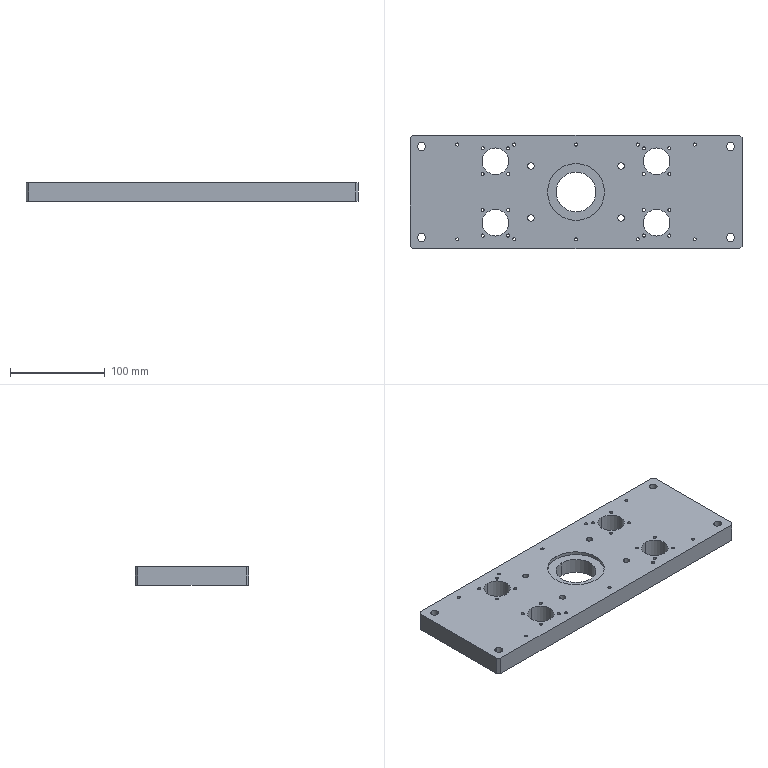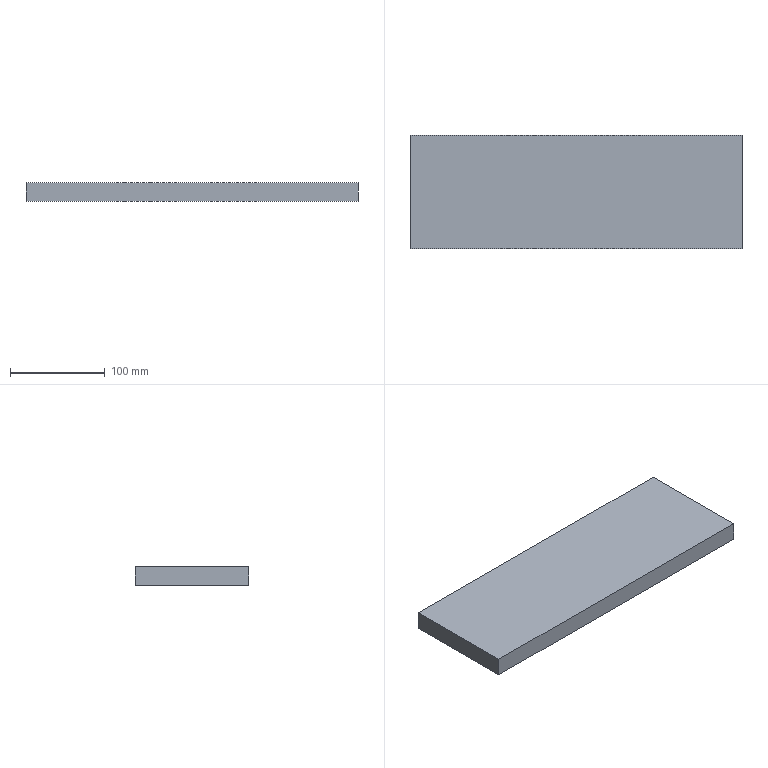CAM job | NX | 3-axis milling, drilling | part box 350 x 120 x 20 mm | stock box 350 x 120 x 20 mm
Tools:
number,name,description,diameter,corner_radius,flute_length,length,flutes
2,D6A45,Milling Tool-5 Parameters,6.0,0.0,3.0,3.0,2
20,ZXZ,Milling Tool-5 Parameters,6.0,0.0,50.0,75.0,2
18,8.5ZT,Drilling Tool,8.5,0.0,35.0,50.0,2
16,6.8ZT,Drilling Tool,6.8,0.0,35.0,50.0,2
13,3.3ZT,Drilling Tool,3.3,0.0,35.0,50.0,2
17,D17R0.8,Milling Tool-5 Parameters,17.0,0.8,50.0,75.0,2
3,D10,Milling Tool-5 Parameters,10.0,0.0,50.0,75.0,2
4,D10JING,Milling Tool-5 Parameters,10.0,0.0,50.0,75.0,2
Operations:
program,operation,operation_type,tool,method,geometry_group,spindle_rpm,surface_speed,feed_per_tooth,feed_cut,feed_plunge,cut_length_mm,path_length_mm,cut_time_min,machine_time_min
1-350-120-20毛胚,DRILLING_COPY_1,Operation,ZXZ,METHOD,A,3000.0,56.0,0.0333,200.0,0.0,156.0,1642.821,0.78,0.9287
1-350-120-20毛胚,DRILLING_COPY_1_COPY_COPY_COPY_COPY,Operation,8.5ZT,METHOD,A,1200.0,33.0,0.0625,150.0,0.0,102.215,791.537,0.6814,0.7504
1-350-120-20毛胚,DRILLING_COPY_1_COPY_COPY_COPY_COPY_COPY_2,Operation,8.5ZT,METHOD,A,1200.0,33.0,0.0625,150.0,0.0,127.768,639.777,0.8518,0.903
1-350-120-20毛胚,DRILLING_COPY_1_COPY_COPY_COPY_COPY_COPY,Operation,6.8ZT,METHOD,A,1200.0,33.0,0.0625,150.0,0.0,100.172,474.554,0.6678,0.7052
1-350-120-20毛胚,DRILLING_COPY_1_COPY_COPY_COPY_COPY_COPY_1,Operation,3.3ZT,METHOD,A,2000.0,20.0,0.025,100.0,0.0,662.777,2252.772,6.628,6.787
1-350-120-20毛胚,HOLE_MILLING,CylinderMilling,D17R0.8,METHOD,A,2000.0,106.0,0.5,2000.0,100.0,12922.078,13623.081,6.461,6.531
1-350-120-20毛胚,HOLE_MILLING_COPY,CylinderMilling,D17R0.8,METHOD,A,2000.0,106.0,0.5,2000.0,100.0,7187.44,7289.44,3.594,3.604
1-350-120-20毛胚,ZLEVEL_PROFILE_1_COPY_COPY_COPY_COPY,ZLevelMilling,D17R0.8,METHOD,A,2000.0,106.0,0.5,2000.0,2000.0,3353.318,4381.405,1.677,1.78
1-350-120-20毛胚,ZLEVEL_PROFILE_COPY_COPY_1_COPY_COPY_COPY_1_COPY,ZLevelMilling,D10JING,METHOD,A,5000.0,157.0,0.1,1000.0,100.0,140.763,1459.596,0.1408,0.2726
1-350-120-20毛胚,FLOOR_WALL_1_COPY_1,VolumeBased25DMillingOperation,D10JING,METHOD,A,5000.0,157.0,0.1,1000.0,100.0,430.906,494.906,0.4309,0.4373
1-350-120-20毛胚,ZLEVEL_PROFILE_COPY_1_COPY_COPY_COPY_COPY_2_COPY,ZLevelMilling,D6A45,METHOD,A,4000.0,75.0,0.125,1000.0,1000.0,1797.244,9299.701,1.797,2.547
1-350-120-20毛胚,ZLEVEL_PROFILE_COPY_1_COPY_COPY_COPY_COPY_2_COPY_COPY,ZLevelMilling,D6A45,METHOD,A,4000.0,75.0,0.125,1000.0,1000.0,129.327,198.327,0.1293,0.1362
1-350-120-20毛胚,刀补4,ZLevelMilling,D10JING,METHOD,A,5000.0,157.0,0.08,800.0,100.0,247.587,973.126,0.3095,0.382
2-350-120-20毛胚,HOLE_MILLING_COPY_1,CylinderMilling,D10,METHOD,B,3000.0,94.0,0.3333,2000.0,100.0,2186.665,2976.506,1.093,1.172
2-350-120-20毛胚,ZLEVEL_PROFILE_COPY_1_COPY_COPY_COPY_COPY_2_COPY_COPY_COPY,ZLevelMilling,D6A45,METHOD,B,4000.0,75.0,0.125,1000.0,1000.0,1831.733,9278.214,1.832,2.576